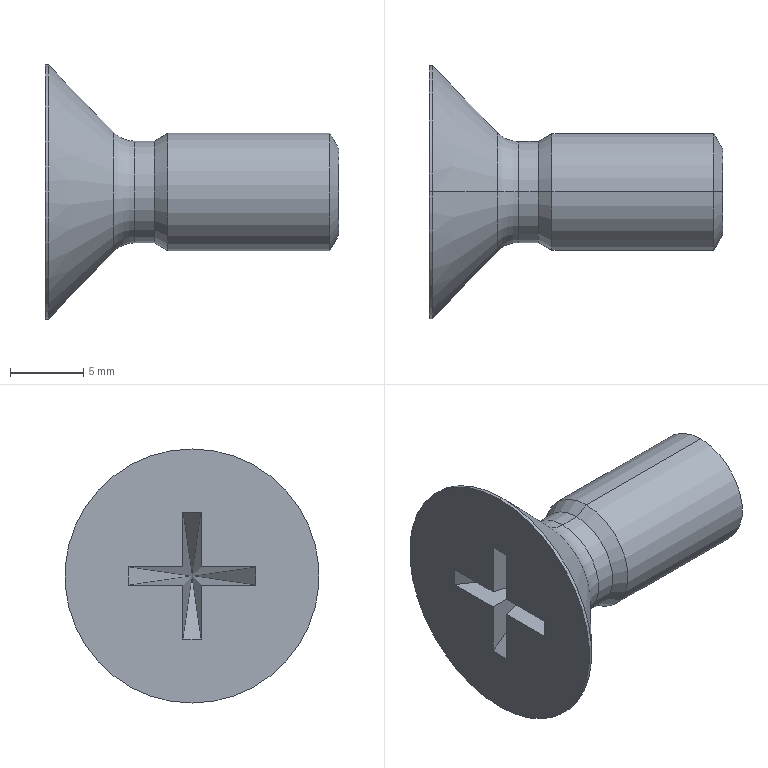Part | SolidWorks | features BaseBody 1 | 1 solid | 28 faces | box 20 x 17.3 x 17.3 mm | volume 1339 mm3 | plane 14 | cone 6 | cylinder 6 | torus 2 | commonest cylinder face diameters 6.928 x2 8 x2 17.3 x2
STEP:
#1=CARTESIAN_POINT('',(0.,4.325,0.625));
#2=VERTEX_POINT('',#1);
#3=CARTESIAN_POINT('',(4.65,0.,0.));
#4=VERTEX_POINT('',#3);
#5=CARTESIAN_POINT('',(0.,4.325,0.625));
#6=DIRECTION('',(0.7287,-0.6778,-0.09795));
#7=VECTOR('',#6,1000.);
#8=LINE('',#5,#7);
#9=EDGE_CURVE('',#2,#4,#8,.T.);
#10=ORIENTED_EDGE('',*,*,#9,.F.);
#11=CARTESIAN_POINT('',(0.,4.325,-0.625));
#12=VERTEX_POINT('',#11);
#13=CARTESIAN_POINT('',(0.,4.325,0.625));
#14=DIRECTION('',(0.,0.,-1.));
#15=VECTOR('',#14,1000.);
#16=LINE('',#13,#15);
#17=EDGE_CURVE('',#2,#12,#16,.T.);
#18=ORIENTED_EDGE('',*,*,#17,.T.);
#19=CARTESIAN_POINT('',(0.,4.325,-0.625));
#20=DIRECTION('',(0.7287,-0.6778,0.09795));
#21=VECTOR('',#20,1000.);
#22=LINE('',#19,#21);
#23=EDGE_CURVE('',#12,#4,#22,.T.);
#24=ORIENTED_EDGE('',*,*,#23,.T.);
#25=EDGE_LOOP('',(#10,#18,#24));
#26=FACE_OUTER_BOUND('',#25,.T.);
#27=CARTESIAN_POINT('',(0.,4.325,0.625));
#28=DIRECTION('',(0.6811,0.7322,0.));
#29=DIRECTION('',(0.,0.,-1.));
#30=AXIS2_PLACEMENT_3D('',#27,#28,#29);
#31=PLANE('',#30);
#32=ADVANCED_FACE('',(#26),#31,.F.);
#33=ORIENTED_EDGE('',*,*,#23,.F.);
#34=CARTESIAN_POINT('',(0.,0.625,-0.625));
#35=VERTEX_POINT('',#34);
#36=CARTESIAN_POINT('',(0.,4.325,-0.625));
#37=DIRECTION('',(0.,-1.,0.));
#38=VECTOR('',#37,1000.);
#39=LINE('',#36,#38);
#40=EDGE_CURVE('',#12,#35,#39,.T.);
#41=ORIENTED_EDGE('',*,*,#40,.T.);
#42=CARTESIAN_POINT('',(4.65,0.,0.));
#43=DIRECTION('',(-0.9824,0.132,-0.132));
#44=VECTOR('',#43,1000.);
#45=LINE('',#42,#44);
#46=EDGE_CURVE('',#4,#35,#45,.T.);
#47=ORIENTED_EDGE('',*,*,#46,.F.);
#48=EDGE_LOOP('',(#33,#41,#47));
#49=FACE_OUTER_BOUND('',#48,.T.);
#50=CARTESIAN_POINT('',(4.65,0.,0.));
#51=DIRECTION('',(-0.1332,0.,0.9911));
#52=DIRECTION('',(0.,1.,0.));
#53=AXIS2_PLACEMENT_3D('',#50,#51,#52);
#54=PLANE('',#53);
#55=ADVANCED_FACE('',(#49),#54,.T.);
#56=CARTESIAN_POINT('',(0.,0.625,0.625));
#57=VERTEX_POINT('',#56);
#58=CARTESIAN_POINT('',(0.,4.325,0.625));
#59=DIRECTION('',(0.,1.,0.));
#60=VECTOR('',#59,1000.);
#61=LINE('',#58,#60);
#62=EDGE_CURVE('',#57,#2,#61,.T.);
#63=ORIENTED_EDGE('',*,*,#62,.T.);
#64=ORIENTED_EDGE('',*,*,#9,.T.);
#65=CARTESIAN_POINT('',(4.65,0.,0.));
#66=DIRECTION('',(0.9824,-0.132,-0.132));
#67=VECTOR('',#66,1000.);
#68=LINE('',#65,#67);
#69=EDGE_CURVE('',#57,#4,#68,.T.);
#70=ORIENTED_EDGE('',*,*,#69,.F.);
#71=EDGE_LOOP('',(#63,#64,#70));
#72=FACE_OUTER_BOUND('',#71,.T.);
#73=CARTESIAN_POINT('',(4.65,0.,0.));
#74=DIRECTION('',(-0.1332,0.,-0.9911));
#75=DIRECTION('',(-0.9911,0.,0.1332));
#76=AXIS2_PLACEMENT_3D('',#73,#74,#75);
#77=PLANE('',#76);
#78=ADVANCED_FACE('',(#72),#77,.T.);
#79=CARTESIAN_POINT('',(0.,-4.325,-0.625));
#80=VERTEX_POINT('',#79);
#81=CARTESIAN_POINT('',(0.,-4.325,-0.625));
#82=DIRECTION('',(0.7287,0.6778,0.09795));
#83=VECTOR('',#82,1000.);
#84=LINE('',#81,#83);
#85=EDGE_CURVE('',#80,#4,#84,.T.);
#86=ORIENTED_EDGE('',*,*,#85,.F.);
#87=CARTESIAN_POINT('',(0.,-4.325,0.625));
#88=VERTEX_POINT('',#87);
#89=CARTESIAN_POINT('',(0.,-4.325,0.625));
#90=DIRECTION('',(0.,0.,1.));
#91=VECTOR('',#90,1000.);
#92=LINE('',#89,#91);
#93=EDGE_CURVE('',#80,#88,#92,.T.);
#94=ORIENTED_EDGE('',*,*,#93,.T.);
#95=CARTESIAN_POINT('',(0.,-4.325,0.625));
#96=DIRECTION('',(0.7287,0.6778,-0.09795));
#97=VECTOR('',#96,1000.);
#98=LINE('',#95,#97);
#99=EDGE_CURVE('',#88,#4,#98,.T.);
#100=ORIENTED_EDGE('',*,*,#99,.T.);
#101=EDGE_LOOP('',(#86,#94,#100));
#102=FACE_OUTER_BOUND('',#101,.T.);
#103=CARTESIAN_POINT('',(0.,-4.325,-0.625));
#104=DIRECTION('',(0.6811,-0.7322,0.));
#105=DIRECTION('',(0.,0.,-1.));
#106=AXIS2_PLACEMENT_3D('',#103,#104,#105);
#107=PLANE('',#106);
#108=ADVANCED_FACE('',(#102),#107,.F.);
#109=CARTESIAN_POINT('',(0.,-0.625,-0.625));
#110=VERTEX_POINT('',#109);
#111=CARTESIAN_POINT('',(0.,4.325,-0.625));
#112=DIRECTION('',(0.,-1.,0.));
#113=VECTOR('',#112,1000.);
#114=LINE('',#111,#113);
#115=EDGE_CURVE('',#110,#80,#114,.T.);
#116=ORIENTED_EDGE('',*,*,#115,.T.);
#117=ORIENTED_EDGE('',*,*,#85,.T.);
#118=CARTESIAN_POINT('',(4.65,0.,0.));
#119=DIRECTION('',(0.9824,0.132,0.132));
#120=VECTOR('',#119,1000.);
#121=LINE('',#118,#120);
#122=EDGE_CURVE('',#110,#4,#121,.T.);
#123=ORIENTED_EDGE('',*,*,#122,.F.);
#124=EDGE_LOOP('',(#116,#117,#123));
#125=FACE_OUTER_BOUND('',#124,.T.);
#126=CARTESIAN_POINT('',(4.65,0.,0.));
#127=DIRECTION('',(-0.1332,0.,0.9911));
#128=DIRECTION('',(0.,1.,0.));
#129=AXIS2_PLACEMENT_3D('',#126,#127,#128);
#130=PLANE('',#129);
#131=ADVANCED_FACE('',(#125),#130,.T.);
#132=ORIENTED_EDGE('',*,*,#99,.F.);
#133=CARTESIAN_POINT('',(0.,-0.625,0.625));
#134=VERTEX_POINT('',#133);
#135=CARTESIAN_POINT('',(0.,4.325,0.625));
#136=DIRECTION('',(0.,1.,0.));
#137=VECTOR('',#136,1000.);
#138=LINE('',#135,#137);
#139=EDGE_CURVE('',#88,#134,#138,.T.);
#140=ORIENTED_EDGE('',*,*,#139,.T.);
#141=CARTESIAN_POINT('',(4.65,0.,0.));
#142=DIRECTION('',(-0.9824,-0.132,0.132));
#143=VECTOR('',#142,1000.);
#144=LINE('',#141,#143);
#145=EDGE_CURVE('',#4,#134,#144,.T.);
#146=ORIENTED_EDGE('',*,*,#145,.F.);
#147=EDGE_LOOP('',(#132,#140,#146));
#148=FACE_OUTER_BOUND('',#147,.T.);
#149=CARTESIAN_POINT('',(4.65,0.,0.));
#150=DIRECTION('',(-0.1332,0.,-0.9911));
#151=DIRECTION('',(-0.9911,0.,0.1332));
#152=AXIS2_PLACEMENT_3D('',#149,#150,#151);
#153=PLANE('',#152);
#154=ADVANCED_FACE('',(#148),#153,.T.);
#155=CARTESIAN_POINT('',(0.,-0.625,4.325));
#156=VERTEX_POINT('',#155);
#157=CARTESIAN_POINT('',(0.,-0.625,4.325));
#158=DIRECTION('',(0.7287,0.09795,-0.6778));
#159=VECTOR('',#158,1000.);
#160=LINE('',#157,#159);
#161=EDGE_CURVE('',#156,#4,#160,.T.);
#162=ORIENTED_EDGE('',*,*,#161,.F.);
#163=CARTESIAN_POINT('',(0.,0.625,4.325));
#164=VERTEX_POINT('',#163);
#165=CARTESIAN_POINT('',(0.,0.625,4.325));
#166=DIRECTION('',(0.,1.,0.));
#167=VECTOR('',#166,1000.);
#168=LINE('',#165,#167);
#169=EDGE_CURVE('',#156,#164,#168,.T.);
#170=ORIENTED_EDGE('',*,*,#169,.T.);
#171=CARTESIAN_POINT('',(0.,0.625,4.325));
#172=DIRECTION('',(0.7287,-0.09795,-0.6778));
#173=VECTOR('',#172,1000.);
#174=LINE('',#171,#173);
#175=EDGE_CURVE('',#164,#4,#174,.T.);
#176=ORIENTED_EDGE('',*,*,#175,.T.);
#177=EDGE_LOOP('',(#162,#170,#176));
#178=FACE_OUTER_BOUND('',#177,.T.);
#179=CARTESIAN_POINT('',(0.,-0.625,4.325));
#180=DIRECTION('',(0.6811,0.,0.7322));
#181=DIRECTION('',(0.,-1.,0.));
#182=AXIS2_PLACEMENT_3D('',#179,#180,#181);
#183=PLANE('',#182);
#184=ADVANCED_FACE('',(#178),#183,.F.);
#185=CARTESIAN_POINT('',(0.,0.625,-4.325));
#186=VERTEX_POINT('',#185);
#187=CARTESIAN_POINT('',(0.,0.625,-4.325));
#188=DIRECTION('',(0.7287,-0.09795,0.6778));
#189=VECTOR('',#188,1000.);
#190=LINE('',#187,#189);
#191=EDGE_CURVE('',#186,#4,#190,.T.);
#192=ORIENTED_EDGE('',*,*,#191,.F.);
#193=CARTESIAN_POINT('',(0.,-0.625,-4.325));
#194=VERTEX_POINT('',#193);
#195=CARTESIAN_POINT('',(0.,0.625,-4.325));
#196=DIRECTION('',(0.,-1.,0.));
#197=VECTOR('',#196,1000.);
#198=LINE('',#195,#197);
#199=EDGE_CURVE('',#186,#194,#198,.T.);
#200=ORIENTED_EDGE('',*,*,#199,.T.);
#201=CARTESIAN_POINT('',(0.,-0.625,-4.325));
#202=DIRECTION('',(0.7287,0.09795,0.6778));
#203=VECTOR('',#202,1000.);
#204=LINE('',#201,#203);
#205=EDGE_CURVE('',#194,#4,#204,.T.);
#206=ORIENTED_EDGE('',*,*,#205,.T.);
#207=EDGE_LOOP('',(#192,#200,#206));
#208=FACE_OUTER_BOUND('',#207,.T.);
#209=CARTESIAN_POINT('',(0.,0.625,-4.325));
#210=DIRECTION('',(0.6811,0.,-0.7322));
#211=DIRECTION('',(0.,-1.,0.));
#212=AXIS2_PLACEMENT_3D('',#209,#210,#211);
#213=PLANE('',#212);
#214=ADVANCED_FACE('',(#208),#213,.F.);
#215=CARTESIAN_POINT('',(20.,0.,2.918));
#216=VERTEX_POINT('',#215);
#217=CARTESIAN_POINT('',(20.,0.,-2.918));
#218=VERTEX_POINT('',#217);
#219=CARTESIAN_POINT('',(20.,0.,0.));
#220=DIRECTION('',(1.,0.,0.));
#221=DIRECTION('',(0.,0.,-1.));
#222=AXIS2_PLACEMENT_3D('',#219,#220,#221);
#223=CIRCLE('',#222,2.917);
#224=EDGE_CURVE('',#216,#218,#223,.T.);
#225=ORIENTED_EDGE('',*,*,#224,.T.);
#226=CARTESIAN_POINT('',(20.,0.,0.));
#227=DIRECTION('',(1.,0.,0.));
#228=DIRECTION('',(0.,0.,-1.));
#229=AXIS2_PLACEMENT_3D('',#226,#227,#228);
#230=CIRCLE('',#229,2.917);
#231=EDGE_CURVE('',#218,#216,#230,.T.);
#232=ORIENTED_EDGE('',*,*,#231,.T.);
#233=EDGE_LOOP('',(#225,#232));
#234=FACE_OUTER_BOUND('',#233,.T.);
#235=CARTESIAN_POINT('',(20.,4.,0.));
#236=DIRECTION('',(-1.,0.,0.));
#237=DIRECTION('',(0.,0.,1.));
#238=AXIS2_PLACEMENT_3D('',#235,#236,#237);
#239=PLANE('',#238);
#240=ADVANCED_FACE('',(#234),#239,.F.);
#241=CARTESIAN_POINT('',(19.382,0.,-4.));
#242=VERTEX_POINT('',#241);
#243=CARTESIAN_POINT('',(19.382,0.,-4.));
#244=DIRECTION('',(-0.4959,0.,-0.8684));
#245=VECTOR('',#244,1000.);
#246=LINE('',#243,#245);
#247=EDGE_CURVE('',#218,#242,#246,.T.);
#248=ORIENTED_EDGE('',*,*,#247,.F.);
#249=ORIENTED_EDGE('',*,*,#224,.F.);
#250=CARTESIAN_POINT('',(19.382,0.,4.));
#251=VERTEX_POINT('',#250);
#252=CARTESIAN_POINT('',(19.382,0.,4.));
#253=DIRECTION('',(-0.4959,0.,0.8684));
#254=VECTOR('',#253,1000.);
#255=LINE('',#252,#254);
#256=EDGE_CURVE('',#216,#251,#255,.T.);
#257=ORIENTED_EDGE('',*,*,#256,.T.);
#258=CARTESIAN_POINT('',(19.382,0.,0.));
#259=DIRECTION('',(1.,0.,0.));
#260=DIRECTION('',(0.,0.,-1.));
#261=AXIS2_PLACEMENT_3D('',#258,#259,#260);
#262=CIRCLE('',#261,4.);
#263=EDGE_CURVE('',#251,#242,#262,.T.);
#264=ORIENTED_EDGE('',*,*,#263,.T.);
#265=EDGE_LOOP('',(#248,#249,#257,#264));
#266=FACE_OUTER_BOUND('',#265,.T.);
#267=CARTESIAN_POINT('',(19.382,0.,0.));
#268=DIRECTION('',(-1.,0.,0.));
#269=DIRECTION('',(0.,0.,1.));
#270=AXIS2_PLACEMENT_3D('',#267,#268,#269);
#271=CONICAL_SURFACE('',#270,4.,1.052);
#272=ADVANCED_FACE('',(#266),#271,.T.);
#273=CARTESIAN_POINT('',(8.365,0.,-4.));
#274=VERTEX_POINT('',#273);
#275=CARTESIAN_POINT('',(0.,0.,-4.));
#276=DIRECTION('',(-1.,0.,0.));
#277=VECTOR('',#276,1000.);
#278=LINE('',#275,#277);
#279=EDGE_CURVE('',#242,#274,#278,.T.);
#280=ORIENTED_EDGE('',*,*,#279,.F.);
#281=ORIENTED_EDGE('',*,*,#263,.F.);
#282=CARTESIAN_POINT('',(8.365,0.,4.));
#283=VERTEX_POINT('',#282);
#284=CARTESIAN_POINT('',(0.,0.,4.));
#285=DIRECTION('',(-1.,0.,0.));
#286=VECTOR('',#285,1000.);
#287=LINE('',#284,#286);
#288=EDGE_CURVE('',#251,#283,#287,.T.);
#289=ORIENTED_EDGE('',*,*,#288,.T.);
#290=CARTESIAN_POINT('',(8.365,0.,0.));
#291=DIRECTION('',(-1.,0.,0.));
#292=DIRECTION('',(0.,0.,1.));
#293=AXIS2_PLACEMENT_3D('',#290,#291,#292);
#294=CIRCLE('',#293,4.);
#295=EDGE_CURVE('',#274,#283,#294,.T.);
#296=ORIENTED_EDGE('',*,*,#295,.F.);
#297=EDGE_LOOP('',(#280,#281,#289,#296));
#298=FACE_OUTER_BOUND('',#297,.T.);
#299=CARTESIAN_POINT('',(0.,0.,0.));
#300=DIRECTION('',(-1.,0.,0.));
#301=DIRECTION('',(0.,0.,1.));
#302=AXIS2_PLACEMENT_3D('',#299,#300,#301);
#303=CYLINDRICAL_SURFACE('',#302,4.);
#304=ADVANCED_FACE('',(#298),#303,.T.);
#305=CARTESIAN_POINT('',(7.436,0.,3.464));
#306=VERTEX_POINT('',#305);
#307=CARTESIAN_POINT('',(8.365,0.,4.));
#308=DIRECTION('',(0.866,0.,0.5));
#309=VECTOR('',#308,1000.);
#310=LINE('',#307,#309);
#311=EDGE_CURVE('',#306,#283,#310,.T.);
#312=ORIENTED_EDGE('',*,*,#311,.F.);
#313=CARTESIAN_POINT('',(7.436,0.,-3.464));
#314=VERTEX_POINT('',#313);
#315=CARTESIAN_POINT('',(7.436,0.,0.));
#316=DIRECTION('',(-1.,0.,0.));
#317=DIRECTION('',(0.,0.,1.));
#318=AXIS2_PLACEMENT_3D('',#315,#316,#317);
#319=CIRCLE('',#318,3.464);
#320=EDGE_CURVE('',#314,#306,#319,.T.);
#321=ORIENTED_EDGE('',*,*,#320,.F.);
#322=CARTESIAN_POINT('',(8.365,0.,-4.));
#323=DIRECTION('',(0.866,0.,-0.5));
#324=VECTOR('',#323,1000.);
#325=LINE('',#322,#324);
#326=EDGE_CURVE('',#314,#274,#325,.T.);
#327=ORIENTED_EDGE('',*,*,#326,.T.);
#328=ORIENTED_EDGE('',*,*,#295,.T.);
#329=EDGE_LOOP('',(#312,#321,#327,#328));
#330=FACE_OUTER_BOUND('',#329,.T.);
#331=CARTESIAN_POINT('',(8.365,0.,0.));
#332=DIRECTION('',(1.,0.,0.));
#333=DIRECTION('',(0.,0.,-1.));
#334=AXIS2_PLACEMENT_3D('',#331,#332,#333);
#335=CONICAL_SURFACE('',#334,4.,0.5236);
#336=ADVANCED_FACE('',(#330),#335,.T.);
#337=CARTESIAN_POINT('',(6.089,0.,-3.464));
#338=VERTEX_POINT('',#337);
#339=CARTESIAN_POINT('',(0.,0.,-3.464));
#340=DIRECTION('',(-1.,0.,0.));
#341=VECTOR('',#340,1000.);
#342=LINE('',#339,#341);
#343=EDGE_CURVE('',#314,#338,#342,.T.);
#344=ORIENTED_EDGE('',*,*,#343,.F.);
#345=ORIENTED_EDGE('',*,*,#320,.T.);
#346=CARTESIAN_POINT('',(6.089,0.,3.464));
#347=VERTEX_POINT('',#346);
#348=CARTESIAN_POINT('',(0.,0.,3.464));
#349=DIRECTION('',(-1.,0.,0.));
#350=VECTOR('',#349,1000.);
#351=LINE('',#348,#350);
#352=EDGE_CURVE('',#306,#347,#351,.T.);
#353=ORIENTED_EDGE('',*,*,#352,.T.);
#354=CARTESIAN_POINT('',(6.089,0.,0.));
#355=DIRECTION('',(-1.,0.,0.));
#356=DIRECTION('',(0.,0.,1.));
#357=AXIS2_PLACEMENT_3D('',#354,#355,#356);
#358=CIRCLE('',#357,3.464);
#359=EDGE_CURVE('',#338,#347,#358,.T.);
#360=ORIENTED_EDGE('',*,*,#359,.F.);
#361=EDGE_LOOP('',(#344,#345,#353,#360));
#362=FACE_OUTER_BOUND('',#361,.T.);
#363=CARTESIAN_POINT('',(0.,0.,0.));
#364=DIRECTION('',(-1.,0.,0.));
#365=DIRECTION('',(0.,0.,1.));
#366=AXIS2_PLACEMENT_3D('',#363,#364,#365);
#367=CYLINDRICAL_SURFACE('',#366,3.464);
#368=ADVANCED_FACE('',(#362),#367,.T.);
#369=CARTESIAN_POINT('',(4.65,0.,-4.075));
#370=VERTEX_POINT('',#369);
#371=CARTESIAN_POINT('',(6.089,0.,-5.464));
#372=DIRECTION('',(0.,1.,0.));
#373=DIRECTION('',(0.,0.,1.));
#374=AXIS2_PLACEMENT_3D('',#371,#372,#373);
#375=CIRCLE('',#374,2.);
#376=EDGE_CURVE('',#370,#338,#375,.T.);
#377=ORIENTED_EDGE('',*,*,#376,.F.);
#378=CARTESIAN_POINT('',(4.65,0.,4.075));
#379=VERTEX_POINT('',#378);
#380=CARTESIAN_POINT('',(4.65,0.,0.));
#381=DIRECTION('',(-1.,0.,0.));
#382=DIRECTION('',(0.,0.,1.));
#383=AXIS2_PLACEMENT_3D('',#380,#381,#382);
#384=CIRCLE('',#383,4.075);
#385=EDGE_CURVE('',#379,#370,#384,.T.);
#386=ORIENTED_EDGE('',*,*,#385,.F.);
#387=CARTESIAN_POINT('',(6.089,0.,5.464));
#388=DIRECTION('',(0.,-1.,0.));
#389=DIRECTION('',(0.,0.,-1.));
#390=AXIS2_PLACEMENT_3D('',#387,#388,#389);
#391=CIRCLE('',#390,2.);
#392=EDGE_CURVE('',#379,#347,#391,.T.);
#393=ORIENTED_EDGE('',*,*,#392,.T.);
#394=CARTESIAN_POINT('',(6.089,0.,0.));
#395=DIRECTION('',(-1.,0.,0.));
#396=DIRECTION('',(0.,0.,1.));
#397=AXIS2_PLACEMENT_3D('',#394,#395,#396);
#398=CIRCLE('',#397,3.464);
#399=EDGE_CURVE('',#347,#338,#398,.T.);
#400=ORIENTED_EDGE('',*,*,#399,.T.);
#401=EDGE_LOOP('',(#377,#386,#393,#400));
#402=FACE_OUTER_BOUND('',#401,.T.);
#403=CARTESIAN_POINT('',(6.089,0.,0.));
#404=DIRECTION('',(-1.,0.,0.));
#405=DIRECTION('',(0.,0.,1.));
#406=AXIS2_PLACEMENT_3D('',#403,#404,#405);
#407=TOROIDAL_SURFACE('',#406,5.464,2.);
#408=ADVANCED_FACE('',(#402),#407,.F.);
#409=CARTESIAN_POINT('',(0.2317,0.,-8.65));
#410=VERTEX_POINT('',#409);
#411=CARTESIAN_POINT('',(4.65,0.,-4.075));
#412=DIRECTION('',(-0.6947,0.,-0.7193));
#413=VECTOR('',#412,1000.);
#414=LINE('',#411,#413);
#415=EDGE_CURVE('',#370,#410,#414,.T.);
#416=ORIENTED_EDGE('',*,*,#415,.F.);
#417=CARTESIAN_POINT('',(4.65,0.,0.));
#418=DIRECTION('',(-1.,0.,0.));
#419=DIRECTION('',(0.,0.,1.));
#420=AXIS2_PLACEMENT_3D('',#417,#418,#419);
#421=CIRCLE('',#420,4.075);
#422=EDGE_CURVE('',#370,#379,#421,.T.);
#423=ORIENTED_EDGE('',*,*,#422,.T.);
#424=CARTESIAN_POINT('',(0.2317,0.,8.65));
#425=VERTEX_POINT('',#424);
#426=CARTESIAN_POINT('',(4.65,0.,4.075));
#427=DIRECTION('',(-0.6947,0.,0.7193));
#428=VECTOR('',#427,1000.);
#429=LINE('',#426,#428);
#430=EDGE_CURVE('',#379,#425,#429,.T.);
#431=ORIENTED_EDGE('',*,*,#430,.T.);
#432=CARTESIAN_POINT('',(0.2317,0.,0.));
#433=DIRECTION('',(-1.,0.,0.));
#434=DIRECTION('',(0.,0.,1.));
#435=AXIS2_PLACEMENT_3D('',#432,#433,#434);
#436=CIRCLE('',#435,8.65);
#437=EDGE_CURVE('',#410,#425,#436,.T.);
#438=ORIENTED_EDGE('',*,*,#437,.F.);
#439=EDGE_LOOP('',(#416,#423,#431,#438));
#440=FACE_OUTER_BOUND('',#439,.T.);
#441=CARTESIAN_POINT('',(4.65,0.,0.));
#442=DIRECTION('',(-1.,0.,0.));
#443=DIRECTION('',(0.,0.,1.));
#444=AXIS2_PLACEMENT_3D('',#441,#442,#443);
#445=CONICAL_SURFACE('',#444,4.075,0.8029);
#446=ADVANCED_FACE('',(#440),#445,.T.);
#447=CARTESIAN_POINT('',(0.,0.,-8.65));
#448=VERTEX_POINT('',#447);
#449=CARTESIAN_POINT('',(0.,0.,-8.65));
#450=DIRECTION('',(-1.,0.,0.));
#451=VECTOR('',#450,1000.);
#452=LINE('',#449,#451);
#453=EDGE_CURVE('',#410,#448,#452,.T.);
#454=ORIENTED_EDGE('',*,*,#453,.F.);
#455=ORIENTED_EDGE('',*,*,#437,.T.);
#456=CARTESIAN_POINT('',(0.,0.,8.65));
#457=VERTEX_POINT('',#456);
#458=CARTESIAN_POINT('',(0.,0.,8.65));
#459=DIRECTION('',(-1.,0.,0.));
#460=VECTOR('',#459,1000.);
#461=LINE('',#458,#460);
#462=EDGE_CURVE('',#425,#457,#461,.T.);
#463=ORIENTED_EDGE('',*,*,#462,.T.);
#464=CARTESIAN_POINT('',(0.,0.,0.));
#465=DIRECTION('',(-1.,0.,0.));
#466=DIRECTION('',(0.,0.,1.));
#467=AXIS2_PLACEMENT_3D('',#464,#465,#466);
#468=CIRCLE('',#467,8.65);
#469=EDGE_CURVE('',#448,#457,#468,.T.);
#470=ORIENTED_EDGE('',*,*,#469,.F.);
#471=EDGE_LOOP('',(#454,#455,#463,#470));
#472=FACE_OUTER_BOUND('',#471,.T.);
#473=CARTESIAN_POINT('',(0.,0.,0.));
#474=DIRECTION('',(-1.,0.,0.));
#475=DIRECTION('',(0.,0.,1.));
#476=AXIS2_PLACEMENT_3D('',#473,#474,#475);
#477=CYLINDRICAL_SURFACE('',#476,8.65);
#478=ADVANCED_FACE('',(#472),#477,.T.);
#479=CARTESIAN_POINT('',(0.,-0.625,-4.325));
#480=DIRECTION('',(0.,0.,1.));
#481=VECTOR('',#480,1000.);
#482=LINE('',#479,#481);
#483=EDGE_CURVE('',#194,#110,#482,.T.);
#484=ORIENTED_EDGE('',*,*,#483,.T.);
#485=ORIENTED_EDGE('',*,*,#122,.T.);
#486=ORIENTED_EDGE('',*,*,#205,.F.);
#487=EDGE_LOOP('',(#484,#485,#486));
#488=FACE_OUTER_BOUND('',#487,.T.);
#489=CARTESIAN_POINT('',(4.65,0.,0.));
#490=DIRECTION('',(-0.1332,0.9911,0.));
#491=DIRECTION('',(0.,0.,1.));
#492=AXIS2_PLACEMENT_3D('',#489,#490,#491);
#493=PLANE('',#492);
#494=ADVANCED_FACE('',(#488),#493,.T.);
#495=ORIENTED_EDGE('',*,*,#161,.T.);
#496=ORIENTED_EDGE('',*,*,#145,.T.);
#497=CARTESIAN_POINT('',(0.,-0.625,-4.325));
#498=DIRECTION('',(0.,0.,1.));
#499=VECTOR('',#498,1000.);
#500=LINE('',#497,#499);
#501=EDGE_CURVE('',#134,#156,#500,.T.);
#502=ORIENTED_EDGE('',*,*,#501,.T.);
#503=EDGE_LOOP('',(#495,#496,#502));
#504=FACE_OUTER_BOUND('',#503,.T.);
#505=CARTESIAN_POINT('',(4.65,0.,0.));
#506=DIRECTION('',(-0.1332,0.9911,0.));
#507=DIRECTION('',(0.,0.,1.));
#508=AXIS2_PLACEMENT_3D('',#505,#506,#507);
#509=PLANE('',#508);
#510=ADVANCED_FACE('',(#504),#509,.T.);
#511=ORIENTED_EDGE('',*,*,#191,.T.);
#512=ORIENTED_EDGE('',*,*,#46,.T.);
#513=CARTESIAN_POINT('',(0.,0.625,-4.325));
#514=DIRECTION('',(0.,0.,-1.));
#515=VECTOR('',#514,1000.);
#516=LINE('',#513,#515);
#517=EDGE_CURVE('',#35,#186,#516,.T.);
#518=ORIENTED_EDGE('',*,*,#517,.T.);
#519=EDGE_LOOP('',(#511,#512,#518));
#520=FACE_OUTER_BOUND('',#519,.T.);
#521=CARTESIAN_POINT('',(4.65,0.,0.));
#522=DIRECTION('',(-0.1332,-0.9911,0.));
#523=DIRECTION('',(-0.9911,0.1332,0.));
#524=AXIS2_PLACEMENT_3D('',#521,#522,#523);
#525=PLANE('',#524);
#526=ADVANCED_FACE('',(#520),#525,.T.);
#527=CARTESIAN_POINT('',(0.,0.625,-4.325));
#528=DIRECTION('',(0.,0.,-1.));
#529=VECTOR('',#528,1000.);
#530=LINE('',#527,#529);
#531=EDGE_CURVE('',#164,#57,#530,.T.);
#532=ORIENTED_EDGE('',*,*,#531,.T.);
#533=ORIENTED_EDGE('',*,*,#69,.T.);
#534=ORIENTED_EDGE('',*,*,#175,.F.);
#535=EDGE_LOOP('',(#532,#533,#534));
#536=FACE_OUTER_BOUND('',#535,.T.);
#537=CARTESIAN_POINT('',(4.65,0.,0.));
#538=DIRECTION('',(-0.1332,-0.9911,0.));
#539=DIRECTION('',(-0.9911,0.1332,0.));
#540=AXIS2_PLACEMENT_3D('',#537,#538,#539);
#541=PLANE('',#540);
#542=ADVANCED_FACE('',(#536),#541,.T.);
#543=ORIENTED_EDGE('',*,*,#62,.F.);
#544=ORIENTED_EDGE('',*,*,#531,.F.);
#545=ORIENTED_EDGE('',*,*,#169,.F.);
#546=ORIENTED_EDGE('',*,*,#501,.F.);
#547=ORIENTED_EDGE('',*,*,#139,.F.);
#548=ORIENTED_EDGE('',*,*,#93,.F.);
#549=ORIENTED_EDGE('',*,*,#115,.F.);
#550=ORIENTED_EDGE('',*,*,#483,.F.);
#551=ORIENTED_EDGE('',*,*,#199,.F.);
#552=ORIENTED_EDGE('',*,*,#517,.F.);
#553=ORIENTED_EDGE('',*,*,#40,.F.);
#554=ORIENTED_EDGE('',*,*,#17,.F.);
#555=EDGE_LOOP('',(#543,#544,#545,#546,#547,#548,#549,#550,#551,#552,#553,#554));
#556=FACE_BOUND('',#555,.T.);
#557=CARTESIAN_POINT('',(0.,0.,0.));
#558=DIRECTION('',(-1.,0.,0.));
#559=DIRECTION('',(0.,0.,1.));
#560=AXIS2_PLACEMENT_3D('',#557,#558,#559);
#561=CIRCLE('',#560,8.65);
#562=EDGE_CURVE('',#457,#448,#561,.T.);
#563=ORIENTED_EDGE('',*,*,#562,.T.);
#564=ORIENTED_EDGE('',*,*,#469,.T.);
#565=EDGE_LOOP('',(#563,#564));
#566=FACE_OUTER_BOUND('',#565,.T.);
#567=CARTESIAN_POINT('',(0.,0.,0.));
#568=DIRECTION('',(1.,0.,0.));
#569=DIRECTION('',(0.,1.,0.));
#570=AXIS2_PLACEMENT_3D('',#567,#568,#569);
#571=PLANE('',#570);
#572=ADVANCED_FACE('',(#556,#566),#571,.F.);
#573=CARTESIAN_POINT('',(0.2317,0.,0.));
#574=DIRECTION('',(-1.,0.,0.));
#575=DIRECTION('',(0.,0.,1.));
#576=AXIS2_PLACEMENT_3D('',#573,#574,#575);
#577=CIRCLE('',#576,8.65);
#578=EDGE_CURVE('',#425,#410,#577,.T.);
#579=ORIENTED_EDGE('',*,*,#578,.T.);
#580=ORIENTED_EDGE('',*,*,#453,.T.);
#581=ORIENTED_EDGE('',*,*,#562,.F.);
#582=ORIENTED_EDGE('',*,*,#462,.F.);
#583=EDGE_LOOP('',(#579,#580,#581,#582));
#584=FACE_OUTER_BOUND('',#583,.T.);
#585=CARTESIAN_POINT('',(0.,0.,0.));
#586=DIRECTION('',(-1.,0.,0.));
#587=DIRECTION('',(0.,0.,1.));
#588=AXIS2_PLACEMENT_3D('',#585,#586,#587);
#589=CYLINDRICAL_SURFACE('',#588,8.65);
#590=ADVANCED_FACE('',(#584),#589,.T.);
#591=ORIENTED_EDGE('',*,*,#385,.T.);
#592=ORIENTED_EDGE('',*,*,#415,.T.);
#593=ORIENTED_EDGE('',*,*,#578,.F.);
#594=ORIENTED_EDGE('',*,*,#430,.F.);
#595=EDGE_LOOP('',(#591,#592,#593,#594));
#596=FACE_OUTER_BOUND('',#595,.T.);
#597=CARTESIAN_POINT('',(4.65,0.,0.));
#598=DIRECTION('',(-1.,0.,0.));
#599=DIRECTION('',(0.,0.,1.));
#600=AXIS2_PLACEMENT_3D('',#597,#598,#599);
#601=CONICAL_SURFACE('',#600,4.075,0.8029);
#602=ADVANCED_FACE('',(#596),#601,.T.);
#603=ORIENTED_EDGE('',*,*,#422,.F.);
#604=ORIENTED_EDGE('',*,*,#376,.T.);
#605=ORIENTED_EDGE('',*,*,#359,.T.);
#606=ORIENTED_EDGE('',*,*,#392,.F.);
#607=EDGE_LOOP('',(#603,#604,#605,#606));
#608=FACE_OUTER_BOUND('',#607,.T.);
#609=CARTESIAN_POINT('',(6.089,0.,0.));
#610=DIRECTION('',(-1.,0.,0.));
#611=DIRECTION('',(0.,0.,1.));
#612=AXIS2_PLACEMENT_3D('',#609,#610,#611);
#613=TOROIDAL_SURFACE('',#612,5.464,2.);
#614=ADVANCED_FACE('',(#608),#613,.F.);
#615=CARTESIAN_POINT('',(7.436,0.,0.));
#616=DIRECTION('',(-1.,0.,0.));
#617=DIRECTION('',(0.,0.,1.));
#618=AXIS2_PLACEMENT_3D('',#615,#616,#617);
#619=CIRCLE('',#618,3.464);
#620=EDGE_CURVE('',#306,#314,#619,.T.);
#621=ORIENTED_EDGE('',*,*,#620,.T.);
#622=ORIENTED_EDGE('',*,*,#343,.T.);
#623=ORIENTED_EDGE('',*,*,#399,.F.);
#624=ORIENTED_EDGE('',*,*,#352,.F.);
#625=EDGE_LOOP('',(#621,#622,#623,#624));
#626=FACE_OUTER_BOUND('',#625,.T.);
#627=CARTESIAN_POINT('',(0.,0.,0.));
#628=DIRECTION('',(-1.,0.,0.));
#629=DIRECTION('',(0.,0.,1.));
#630=AXIS2_PLACEMENT_3D('',#627,#628,#629);
#631=CYLINDRICAL_SURFACE('',#630,3.464);
#632=ADVANCED_FACE('',(#626),#631,.T.);
#633=ORIENTED_EDGE('',*,*,#620,.F.);
#634=ORIENTED_EDGE('',*,*,#311,.T.);
#635=CARTESIAN_POINT('',(8.365,0.,0.));
#636=DIRECTION('',(-1.,0.,0.));
#637=DIRECTION('',(0.,0.,1.));
#638=AXIS2_PLACEMENT_3D('',#635,#636,#637);
#639=CIRCLE('',#638,4.);
#640=EDGE_CURVE('',#283,#274,#639,.T.);
#641=ORIENTED_EDGE('',*,*,#640,.T.);
#642=ORIENTED_EDGE('',*,*,#326,.F.);
#643=EDGE_LOOP('',(#633,#634,#641,#642));
#644=FACE_OUTER_BOUND('',#643,.T.);
#645=CARTESIAN_POINT('',(8.365,0.,0.));
#646=DIRECTION('',(1.,0.,0.));
#647=DIRECTION('',(0.,0.,-1.));
#648=AXIS2_PLACEMENT_3D('',#645,#646,#647);
#649=CONICAL_SURFACE('',#648,4.,0.5236);
#650=ADVANCED_FACE('',(#644),#649,.T.);
#651=CARTESIAN_POINT('',(19.382,0.,0.));
#652=DIRECTION('',(1.,0.,0.));
#653=DIRECTION('',(0.,0.,-1.));
#654=AXIS2_PLACEMENT_3D('',#651,#652,#653);
#655=CIRCLE('',#654,4.);
#656=EDGE_CURVE('',#242,#251,#655,.T.);
#657=ORIENTED_EDGE('',*,*,#656,.F.);
#658=ORIENTED_EDGE('',*,*,#279,.T.);
#659=ORIENTED_EDGE('',*,*,#640,.F.);
#660=ORIENTED_EDGE('',*,*,#288,.F.);
#661=EDGE_LOOP('',(#657,#658,#659,#660));
#662=FACE_OUTER_BOUND('',#661,.T.);
#663=CARTESIAN_POINT('',(0.,0.,0.));
#664=DIRECTION('',(-1.,0.,0.));
#665=DIRECTION('',(0.,0.,1.));
#666=AXIS2_PLACEMENT_3D('',#663,#664,#665);
#667=CYLINDRICAL_SURFACE('',#666,4.);
#668=ADVANCED_FACE('',(#662),#667,.T.);
#669=ORIENTED_EDGE('',*,*,#231,.F.);
#670=ORIENTED_EDGE('',*,*,#247,.T.);
#671=ORIENTED_EDGE('',*,*,#656,.T.);
#672=ORIENTED_EDGE('',*,*,#256,.F.);
#673=EDGE_LOOP('',(#669,#670,#671,#672));
#674=FACE_OUTER_BOUND('',#673,.T.);
#675=CARTESIAN_POINT('',(19.382,0.,0.));
#676=DIRECTION('',(-1.,0.,0.));
#677=DIRECTION('',(0.,0.,1.));
#678=AXIS2_PLACEMENT_3D('',#675,#676,#677);
#679=CONICAL_SURFACE('',#678,4.,1.052);
#680=ADVANCED_FACE('',(#674),#679,.T.);
#681=CLOSED_SHELL('',(#32,#55,#78,#108,#131,#154,#184,#214,#240,#272,#304,#336,#368,#408,#446,#478,#494,#510,#526,#542,#572,#590,#602,#614,#632,#650,#668,#680));
#682=MANIFOLD_SOLID_BREP('',#681);
#683=CARTESIAN_POINT('',(0.,0.,0.));
#684=DIRECTION('',(0.,0.,1.));
#685=DIRECTION('',(1.,0.,0.));
#686=AXIS2_PLACEMENT_3D('',#683,#684,#685);
#687=(LENGTH_UNIT()NAMED_UNIT(*)SI_UNIT(.MILLI.,.METRE.));
#688=UNCERTAINTY_MEASURE_WITH_UNIT(LENGTH_MEASURE(0.00001),#687,'','');
#689=(NAMED_UNIT(*)PLANE_ANGLE_UNIT()SI_UNIT($,.RADIAN.));
#690=(NAMED_UNIT(*)SI_UNIT($,.STERADIAN.)SOLID_ANGLE_UNIT());
#691=(GEOMETRIC_REPRESENTATION_CONTEXT(3)GLOBAL_UNCERTAINTY_ASSIGNED_CONTEXT((#688))GLOBAL_UNIT_ASSIGNED_CONTEXT((#687,#689,#690))REPRESENTATION_CONTEXT('',''));
#692=ADVANCED_BREP_SHAPE_REPRESENTATION('',(#682,#686),#691);